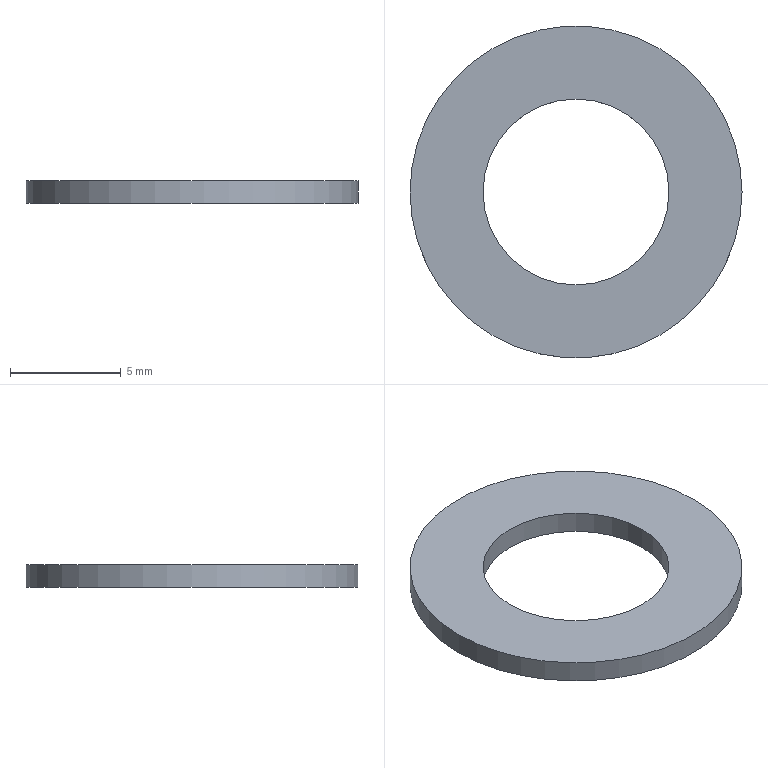Part | NX | features DATUM_CSYS 2, EXTRUDE 1, SKETCH 1 | 1 solid | 4 faces | box 15 x 15 x 1 mm | volume 121.297 mm3 | cylinder 2 | plane 2 | commonest cylinder face diameters 8.4 x1 15 x1
STEP:
#1=CARTESIAN_POINT('',(7.5,0.,0.5));
#2=VERTEX_POINT('',#1);
#3=CARTESIAN_POINT('',(0.,0.,0.5));
#4=DIRECTION('',(0.,0.,1.));
#5=DIRECTION('',(1.,0.,0.));
#6=AXIS2_PLACEMENT_3D('',#3,#4,#5);
#7=CIRCLE('',#6,7.5);
#8=EDGE_CURVE('',#2,#2,#7,.T.);
#9=ORIENTED_EDGE('',*,*,#8,.F.);
#10=EDGE_LOOP('',(#9));
#11=FACE_BOUND('',#10,.T.);
#12=CARTESIAN_POINT('',(7.5,0.,-0.5));
#13=VERTEX_POINT('',#12);
#14=CARTESIAN_POINT('',(0.,0.,-0.5));
#15=DIRECTION('',(0.,0.,1.));
#16=DIRECTION('',(1.,0.,0.));
#17=AXIS2_PLACEMENT_3D('',#14,#15,#16);
#18=CIRCLE('',#17,7.5);
#19=EDGE_CURVE('',#13,#13,#18,.T.);
#20=ORIENTED_EDGE('',*,*,#19,.T.);
#21=EDGE_LOOP('',(#20));
#22=FACE_BOUND('',#21,.T.);
#23=CARTESIAN_POINT('',(0.,0.,0.5));
#24=DIRECTION('',(0.,0.,-1.));
#25=DIRECTION('',(-1.,0.,0.));
#26=AXIS2_PLACEMENT_3D('',#23,#24,#25);
#27=CYLINDRICAL_SURFACE('',#26,7.5);
#28=ADVANCED_FACE('',(#11,#22),#27,.T.);
#29=CARTESIAN_POINT('',(4.2,0.,0.5));
#30=VERTEX_POINT('',#29);
#31=CARTESIAN_POINT('',(0.,0.,0.5));
#32=DIRECTION('',(0.,0.,1.));
#33=DIRECTION('',(1.,0.,0.));
#34=AXIS2_PLACEMENT_3D('',#31,#32,#33);
#35=CIRCLE('',#34,4.2);
#36=EDGE_CURVE('',#30,#30,#35,.T.);
#37=ORIENTED_EDGE('',*,*,#36,.T.);
#38=EDGE_LOOP('',(#37));
#39=FACE_BOUND('',#38,.T.);
#40=CARTESIAN_POINT('',(4.2,0.,-0.5));
#41=VERTEX_POINT('',#40);
#42=CARTESIAN_POINT('',(0.,0.,-0.5));
#43=DIRECTION('',(0.,0.,1.));
#44=DIRECTION('',(1.,0.,0.));
#45=AXIS2_PLACEMENT_3D('',#42,#43,#44);
#46=CIRCLE('',#45,4.2);
#47=EDGE_CURVE('',#41,#41,#46,.T.);
#48=ORIENTED_EDGE('',*,*,#47,.F.);
#49=EDGE_LOOP('',(#48));
#50=FACE_BOUND('',#49,.T.);
#51=CARTESIAN_POINT('',(0.,0.,0.5));
#52=DIRECTION('',(0.,0.,-1.));
#53=DIRECTION('',(-1.,0.,0.));
#54=AXIS2_PLACEMENT_3D('',#51,#52,#53);
#55=CYLINDRICAL_SURFACE('',#54,4.2);
#56=ADVANCED_FACE('',(#39,#50),#55,.F.);
#57=ORIENTED_EDGE('',*,*,#8,.T.);
#58=EDGE_LOOP('',(#57));
#59=FACE_BOUND('',#58,.T.);
#60=ORIENTED_EDGE('',*,*,#36,.F.);
#61=EDGE_LOOP('',(#60));
#62=FACE_BOUND('',#61,.T.);
#63=CARTESIAN_POINT('',(0.,0.,0.5));
#64=DIRECTION('',(0.,0.,1.));
#65=DIRECTION('',(1.,0.,0.));
#66=AXIS2_PLACEMENT_3D('',#63,#64,#65);
#67=PLANE('',#66);
#68=ADVANCED_FACE('',(#59,#62),#67,.T.);
#69=ORIENTED_EDGE('',*,*,#19,.F.);
#70=EDGE_LOOP('',(#69));
#71=FACE_BOUND('',#70,.T.);
#72=ORIENTED_EDGE('',*,*,#47,.T.);
#73=EDGE_LOOP('',(#72));
#74=FACE_BOUND('',#73,.T.);
#75=CARTESIAN_POINT('',(0.,0.,-0.5));
#76=DIRECTION('',(0.,0.,1.));
#77=DIRECTION('',(1.,0.,0.));
#78=AXIS2_PLACEMENT_3D('',#75,#76,#77);
#79=PLANE('',#78);
#80=ADVANCED_FACE('',(#71,#74),#79,.F.);
#81=CLOSED_SHELL('',(#28,#56,#68,#80));
#82=MANIFOLD_SOLID_BREP('',#81);
#83=(LENGTH_UNIT()NAMED_UNIT(*)SI_UNIT(.MILLI.,.METRE.));
#84=UNCERTAINTY_MEASURE_WITH_UNIT(LENGTH_MEASURE(0.00001),#83,'','');
#85=(NAMED_UNIT(*)PLANE_ANGLE_UNIT()SI_UNIT($,.RADIAN.));
#86=(NAMED_UNIT(*)SI_UNIT($,.STERADIAN.)SOLID_ANGLE_UNIT());
#87=(GEOMETRIC_REPRESENTATION_CONTEXT(3)GLOBAL_UNCERTAINTY_ASSIGNED_CONTEXT((#84))GLOBAL_UNIT_ASSIGNED_CONTEXT((#83,#85,#86))REPRESENTATION_CONTEXT('',''));
#88=ADVANCED_BREP_SHAPE_REPRESENTATION('',(#82),#87);